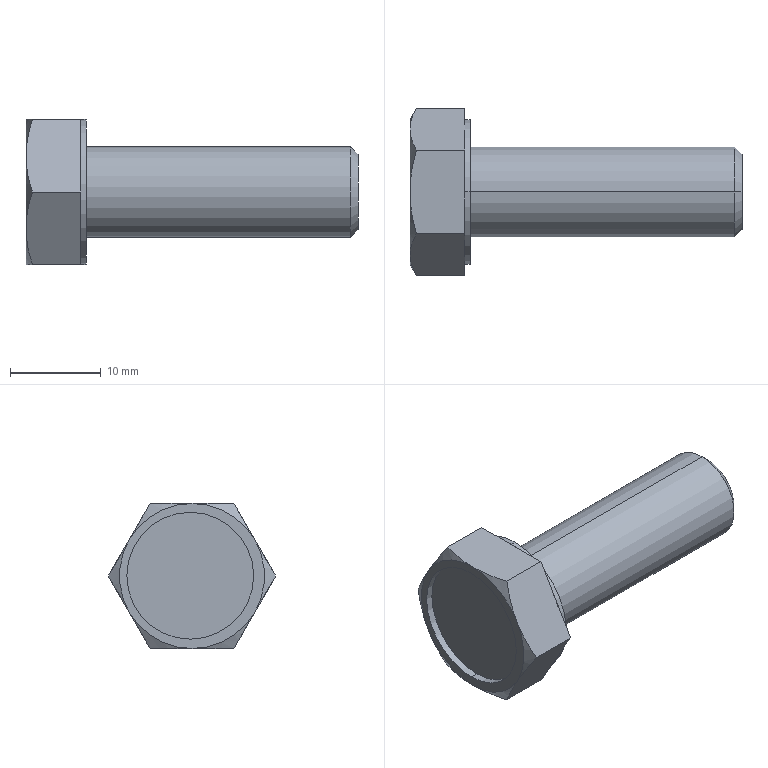Part | STEP file | formed hex screw_am_B18.2.3.2M - Formed hex screw, M10 x 1.5 x 30 --30WN | 1 solid | 30 faces | box 36.63 x 18.475 x 16 mm | volume 3671 mm3 | plane 16 | cone 8 | cylinder 6 | commonest cylinder face diameters 10 x2 14 x2 16 x2